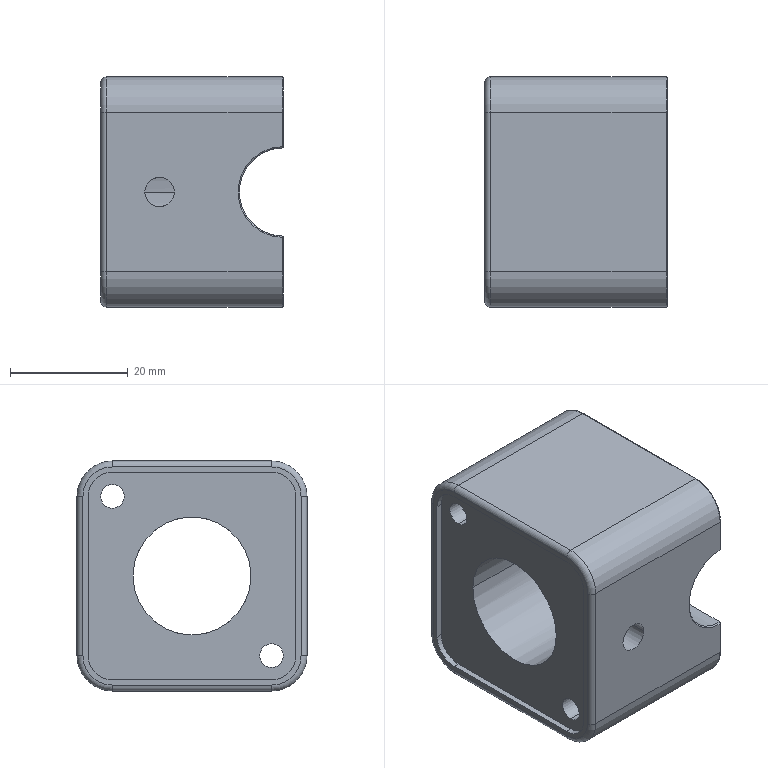NC program | NX | posted with a generic post | part box 31 x 39 x 39 mm
Whole program:
N10 G17 G21 G94 G90
(FACE_MILLING , TOOL : D50面刀)
N12 T01 M6
N14 G54
N16 G17 G0 G90 X-67.6 Y0. S3500 M3
N18 G43 Z13. H1
N20 Z3.
N22 G94 G1 Z0. F480.
N24 X-42.6
N26 X42.6 F800.
N28 X67.6
N30 Z3.
N32 G0 Z13.
N34 M5
(ADAPTIVE_MILLING , TOOL : D12C)
N36 T02 M6
N38 G54
N40 G17 G0 G90 X-31.788 Y-0.055 S6500 M3
N42 G43 Z10.1 H2
N44 Z-29.
N46 G94 G1 Z-32. F1200.
N48 X-30.034 Y-0.606 F2000.
N50 G3 X-28.621 Y-0.055 R1.22
N52 X-27.902 Y2.503 R6.631
N54 X-27.53 Y11.115 R77.337
N56 G2 X-27.476 Y19.739 R652.011
N58 X-24.339 Y24.645 R7.121
N60 X-18.3 Y26.893 R14.361
N62 X-9.325 Y27.446 R63.764
N64 G1 X-8.2 Y27.458
N66 X-7.075 Y27.467
N68 X-5.45 Y27.474
N70 X-3.45 Y27.48
N72 X-0.325 Y27.483
N74 X5.925 Y27.484
N76 X19.175 Y27.482
N78 X19.3 Y27.481
N80 X19.425 Y27.477
N82 X19.55 Y27.471
N84 X19.675 Y27.46
N86 G2 X24.607 Y24.368 R7.095
N88 X26.884 Y18.34 R14.24
N90 X27.443 Y9.741 R59.794
N92 G1 X27.454 Y8.866
N94 X27.465 Y7.741
N96 X27.473 Y6.491
N98 X27.48 Y4.741
N100 X27.485 Y2.491
N102 X27.488 Y-1.384
N104 X27.489 Y-11.509
N106 Y-19.259
N108 X27.485 Y-19.383
N110 X27.479 Y-19.508
N112 X27.47 Y-19.633
N114 G2 X24.401 Y-24.579 R7.07
N116 X18.256 Y-26.89 R14.307
N118 X9.906 Y-27.432 R59.459
N120 G1 X8.906 Y-27.445
N122 X7.781 Y-27.456
N124 X6.406 Y-27.465
N126 X4.656 Y-27.472
N128 X2.156 Y-27.477
N130 X-1.719 Y-27.48
N132 X-12.969 Y-27.481
N134 X-19.219 Y-27.482
N136 X-19.344 Y-27.48
N138 X-19.469 Y-27.474
N140 X-19.593 Y-27.466
N142 G2 X-24.482 Y-24.531 R6.979
N144 X-26.869 Y-18.418 R13.923
N146 X-27.442 Y-9.57 R60.624
N148 X-27.394 Y-2.323 R91.496
N150 G3 X-26.539 Y13.769 R130.767
N152 G2 X-26.388 Y17.386 R22.547
N154 X-21.818 Y23.656 R9.393
N156 X-14.847 Y25.904 R18.303
N158 X-4.743 Y26.438 R83.08
N160 G1 X-3.618 Y26.448
N162 X-2.118 Y26.457
N164 X-0.243 Y26.464
N166 X2.257 Y26.469
N168 X6.257 Y26.472
N170 X15.882
N172 G2 X23.312 Y22.305 R9.011
N174 X25.832 Y15.306 R16.91
N176 X26.435 Y5.208 R73.872
N178 G1 X26.448 Y3.958
N180 X26.457 Y2.708
N182 X26.465 Y1.083
N184 X26.471 Y-1.042
N186 X26.476 Y-4.042
N188 X26.478 Y-9.667
N190 G2 X26.439 Y-16.666 R198.924
N192 X22.175 Y-23.4 R9.126
N194 X15.149 Y-25.851 R17.286
N196 X5.048 Y-26.428 R76.941
N198 G1 X3.923 Y-26.439
N200 X2.549 Y-26.449
N202 X0.924 Y-26.457
N204 X-1.201 Y-26.463
N206 X-4.326 Y-26.468
N208 X-10.201 Y-26.47
N210 G2 X-16.7 Y-26.429 R163.076
N212 X-23.422 Y-22.143 R9.144
N214 X-25.842 Y-15.237 R17.24
N216 X-26.04 Y0.726 R70.302
N218 G3 X-25.583 Y13.777 R171.534
N220 G2 X-24.847 Y17.688 R13.664
N222 X-22.73 Y21.317 R13.93
N224 X-19.5 Y24.002 R13.93
N226 X-15.546 Y25.421 R13.93
N228 G1 X-13.527 Y25.598
N230 X-13.472 Y25.6
N232 X13.472
N234 X13.527 Y25.598
N236 G2 X17.585 Y24.885 R14.157
N238 X21.317 Y22.73 R13.76
N240 X24.002 Y19.5 R13.93
N242 X25.421 Y15.546 R13.93
N244 G1 X25.598 Y13.527
N246 X25.6 Y13.472
N248 Y-13.472
N250 X25.598 Y-13.527
N252 G2 X24.885 Y-17.585 R14.157
N254 X22.73 Y-21.317 R13.76
N256 X19.5 Y-24.002 R13.93
N258 X15.546 Y-25.421 R13.93
N260 G1 X13.527 Y-25.598
N262 X13.472 Y-25.6
N264 X-13.472
N266 X-13.527 Y-25.598
N268 G2 X-17.585 Y-24.885 R14.157
N270 X-21.317 Y-22.73 R13.76
N272 X-24.002 Y-19.5 R13.93
N274 X-25.421 Y-15.546 R13.93
N276 G1 X-25.598 Y-13.527
N278 X-25.6 Y-13.472
N280 Y13.472
N282 X-25.598 Y13.527
N284 X-25.5 Y14.648
N286 G3 X-26.643 Y15.964 R1.217
N288 G1 X-28.366 Y16.056
N290 Z-29.
N292 G0 Z10.1
(HOLE_MILLING , TOOL : D12C)
N294 X0. Y0.
N296 Z10.
N298 Z0.5
N300 G3 X1.9 Y1.9 R1.9 F300.
N302 X0. Y3.8 R1.9
N304 X0. Y3.8 Z-0.5 I0. J-3.8 F500.
N306 X0. Y3.8 Z-1.5 I0. J-3.8
N308 X0. Y3.8 Z-2.5 I0. J-3.8
N310 X0. Y3.8 Z-3.5 I0. J-3.8
N312 X0. Y3.8 Z-4.5 I0. J-3.8
N314 X0. Y3.8 Z-5.5 I0. J-3.8
N316 X0. Y3.8 Z-6.5 I0. J-3.8
N318 X0. Y3.8 Z-7.5 I0. J-3.8
N320 X0. Y3.8 Z-8.5 I0. J-3.8
N322 X0. Y3.8 Z-9.5 I0. J-3.8
N324 X0. Y3.8 Z-10.5 I0. J-3.8
N326 X0. Y3.8 Z-11.5 I0. J-3.8
N328 X0. Y3.8 Z-12.5 I0. J-3.8
N330 X0. Y3.8 Z-13.5 I0. J-3.8
N332 X0. Y3.8 Z-14.5 I0. J-3.8
N334 X0. Y3.8 Z-15.5 I0. J-3.8
N336 X0. Y3.8 Z-16.5 I0. J-3.8
N338 X0. Y3.8 Z-17.5 I0. J-3.8
N340 X0. Y3.8 Z-18.5 I0. J-3.8
N342 X0. Y3.8 Z-19.5 I0. J-3.8
N344 X0. Y3.8 Z-20.5 I0. J-3.8
N346 X0. Y3.8 Z-21.5 I0. J-3.8
N348 X0. Y3.8 Z-22.5 I0. J-3.8
N350 X0. Y3.8 Z-23.5 I0. J-3.8
N352 X0. Y3.8 Z-24.5 I0. J-3.8
N354 X0. Y3.8 Z-25.5 I0. J-3.8
N356 X0. Y3.8 Z-26.5 I0. J-3.8
N358 X0. Y3.8 Z-27.5 I0. J-3.8
N360 X0. Y3.8 Z-28.5 I0. J-3.8
N362 X0. Y3.8 Z-29.5 I0. J-3.8
N364 X0. Y3.8 Z-30.5 I0. J-3.8
N366 X0. Y3.8 Z-31.5 I0. J-3.8
N368 X-3.8 Y0. R3.8
N370 X0. Y3.8 R-3.8
N372 X-1.9 Y1.9 R1.9
N374 X0. Y0. R1.9
N376 G0 Z10.
(PLANAR_PROFILE , TOOL : D12C)
N378 X-28.5 Y-16.5 S3500
N380 Z-29.
N382 G1 Z-32. F800.
N384 G3 X-25.5 Y-13.5 R3.
N386 G1 Y13.5
N388 G2 X-13.5 Y25.5 R12.
N390 G1 X13.5
N392 G2 X25.5 Y13.5 R12.
N394 G1 Y-13.5
N396 G2 X13.5 Y-25.5 R12.
N398 G1 X-13.5
N400 G2 X-25.5 Y-13.5 R12.
N402 G3 X-28.5 Y-10.5 R3.
N404 G1 Z-29.
N406 G0 Z10.
(PLANAR_PROFILE_COPY , TOOL : D12C)
N408 X-1. Y-2.828 S4500
N410 Z-30.
N412 G1 Z-32. F300.
N414 Y-3.
N416 G3 X0. Y-4. R1.
N418 X4. Y0. R4.
N420 X0. Y-4. R-4.
N422 X1. Y-3. R1.
N424 G1 Y-2.828
N426 Z-30.
N428 G0 Z10.
N430 M5
(PLANAR_PROFILE_COPY_COPY , TOOL : D10点钻)
N432 T03 M6
N434 G54
N436 G17 G0 G90 X-1. Y-7.433 S3500 M3
N438 G43 Z10. H3
N440 Z0.5
N442 G94 G1 Z-1.5 F800.
N444 Y-7.5
N446 G3 X0. Y-8.5 R1.
N448 X8.5 Y0. R8.5
N450 X0. Y-8.5 R-8.5
N452 X1. Y-7.433 R1.002
N454 G1 Z0.5
N456 G0 Z10.
(DRILLING , TOOL : D10点钻)
N458 S1200
N460 X-13.5 Y13.5
N462 G43 Z3. H3
N464 G81 G99 Z-3.6 F250. R3.
N466 X13.5 Y-13.5
N468 G80
(DRILLING_COPY , TOOL : D10点钻)
N470 G81 X-13.5 Y-13.5 Z-2. F250. R3.
N472 X13.5 Y13.5
N474 G80
N476 M5
(DRILLING_COPY_1 , TOOL : D4.2钻头)
N478 T04 M6
N480 G54
N482 G17 G43 G0 G90 X-13.5 Y13.5 S2000 H4 M3
N484 Z3.
N486 G94 G83 G99 Z-33. F250. Q3. R3.
N488 X13.5 Y-13.5
N490 G80
N492 M5
(DRILLING_COPY_COPY , TOOL : D3.3钻头)
N494 T05 M6
N496 G54
N498 G17 G0 G90 X-13.5 Y-13.5 S1200 M3
N500 G43 Z3. H5
N502 G94 G81 G99 Z-11.5 F250. R3.
N504 X13.5 Y13.5
N506 G80
N508 M5
(HOLE_MILLING_1 , TOOL : D5精刀)
N510 T07 M6
N512 G54
N514 G17 G0 G90 X-13.5 Y13.5 S4500 M3
N516 G43 Z10. H7
N518 Z0.3
N520 G94 G3 X-12.95 Y14.05 R0.55 F800.
N522 X-13.5 Y14.6 R0.55
N524 X-13.5 Y14.6 Z-0.2 I0. J-1.1
N526 X-13.5 Y14.6 Z-0.7 I0. J-1.1
N528 X-13.5 Y14.6 Z-1.2 I0. J-1.1
N530 X-13.5 Y14.6 Z-1.7 I0. J-1.1
N532 X-13.5 Y14.6 Z-2.2 I0. J-1.1
N534 X-13.5 Y14.6 Z-2.7 I0. J-1.1
N536 X-13.5 Y14.6 Z-3.2 I0. J-1.1
N538 X-13.5 Y14.6 Z-3.7 I0. J-1.1
N540 X-13.5 Y14.6 Z-4.2 I0. J-1.1
N542 X-13.5 Y14.6 Z-4.7 I0. J-1.1
N544 X-13.5 Y14.6 Z-5.2 I0. J-1.1
N546 X-13.5 Y14.6 Z-5.7 I0. J-1.1
N548 X-13.5 Y14.6 Z-6.2 I0. J-1.1
N550 X-13.5 Y14.6 Z-6.7 I0. J-1.1
N552 X-13.5 Y14.6 Z-7.2 I0. J-1.1
N554 X-13.5 Y14.6 Z-7.7 I0. J-1.1
N556 X-13.5 Y14.6 Z-8.2 I0. J-1.1
N558 X-13.5 Y14.6 Z-8.7 I0. J-1.1
N560 X-13.5 Y14.6 Z-9.2 I0. J-1.1
N562 X-13.5 Y14.6 Z-9.7 I0. J-1.1
N564 X-12.853 Y12.61 Z-10. R-1.1
N566 X-12.61 Y14.147 R1.1
N568 X-12.853 Y12.61 R-1.1
N570 X-12.732 Y13.378 R0.55
N572 X-13.5 Y13.5 R0.55
N574 G0 Z10.
N576 X13.5 Y-13.5
N578 Z0.3
N580 G3 X14.05 Y-12.95 R0.55
N582 X13.5 Y-12.4 R0.55
N584 X13.5 Y-12.4 Z-0.2 I0. J-1.1
N586 X13.5 Y-12.4 Z-0.7 I0. J-1.1
N588 X13.5 Y-12.4 Z-1.2 I0. J-1.1
N590 X13.5 Y-12.4 Z-1.7 I0. J-1.1
N592 X13.5 Y-12.4 Z-2.2 I0. J-1.1
N594 X13.5 Y-12.4 Z-2.7 I0. J-1.1
N596 X13.5 Y-12.4 Z-3.2 I0. J-1.1
N598 X13.5 Y-12.4 Z-3.7 I0. J-1.1
N600 X13.5 Y-12.4 Z-4.2 I0. J-1.1
N602 X13.5 Y-12.4 Z-4.7 I0. J-1.1
N604 X13.5 Y-12.4 Z-5.2 I0. J-1.1
N606 X13.5 Y-12.4 Z-5.7 I0. J-1.1
N608 X13.5 Y-12.4 Z-6.2 I0. J-1.1
N610 X13.5 Y-12.4 Z-6.7 I0. J-1.1
N612 X13.5 Y-12.4 Z-7.2 I0. J-1.1
N614 X13.5 Y-12.4 Z-7.7 I0. J-1.1
N616 X13.5 Y-12.4 Z-8.2 I0. J-1.1
N618 X13.5 Y-12.4 Z-8.7 I0. J-1.1
N620 X13.5 Y-12.4 Z-9.2 I0. J-1.1
N622 X13.5 Y-12.4 Z-9.7 I0. J-1.1
N624 X14.147 Y-14.39 Z-10. R-1.1
N626 X14.39 Y-12.853 R1.1
N628 X14.147 Y-14.39 R-1.1
N630 X14.268 Y-13.622 R0.55
N632 X13.5 Y-13.5 R0.55
N634 G0 Z10.
N636 M5
(ZLEVEL_PROFILE , TOOL : R0.5)
N638 T08 M6
N640 G54
N642 G17 G0 G90 X-7.084 Y-19.774 S4500 M3
N644 G43 Z10. H8
N646 Z2.98
N648 G94 G1 Z-0.02 F1500.
N650 G3 X-7.546 Y-19.466 R0.5
N652 G1 X-13.5
N654 G2 X-19.466 Y-13.5 R5.966
N656 G1 Y13.5
N658 G2 X-13.5 Y19.466 R5.966
N660 G1 X-7.546
N662 X-7.555 Y19.502 Z-0.03
N664 X-7.564 Y19.533 Z-0.04
N666 X-13.5
N668 G3 X-19.533 Y13.5 R6.033
N670 G1 Y-13.5
N672 G3 X-13.5 Y-19.533 R6.033
N674 G1 X-7.564
N676 X-7.571 Y-19.56 Z-0.05
N678 X-7.578 Y-19.584 Z-0.06
N680 X-13.5
N682 G2 X-19.584 Y-13.5 R6.084
N684 G1 Y13.5
N686 G2 X-13.5 Y19.584 R6.084
N688 G1 X-7.578
N690 X-7.583 Y19.605 Z-0.07
N692 X-7.589 Y19.625 Z-0.08
N694 X-13.5
N696 G3 X-19.625 Y13.5 R6.125
N698 G1 Y-13.5
N700 G3 X-13.5 Y-19.625 R6.125
N702 G1 X-7.589
N704 X-7.598 Y-19.661 Z-0.1
N706 X-13.5
N708 G2 X-19.661 Y-13.5 R6.161
N710 G1 Y13.5
N712 G2 X-13.5 Y19.661 R6.161
N714 G1 X-7.598
N716 X-7.607 Y19.692 Z-0.12
N718 X-13.5
N720 G3 X-19.692 Y13.5 R6.192
N722 G1 Y-13.5
N724 G3 X-13.5 Y-19.692 R6.192
N726 G1 X-7.607
N728 X-7.615 Y-19.72 Z-0.14
N730 X-13.5
N732 G2 X-19.72 Y-13.5 R6.22
N734 G1 Y13.5
N736 G2 X-13.5 Y19.72 R6.22
N738 G1 X-7.615
N740 X-7.621 Y19.745 Z-0.16
N742 X-13.5
N744 G3 X-19.745 Y13.5 R6.245
N746 G1 Y-13.5
N748 G3 X-13.5 Y-19.745 R6.245
N750 G1 X-7.621
N752 X-7.628 Y-19.769 Z-0.18
N754 X-13.5
N756 G2 X-19.769 Y-13.5 R6.269
N758 G1 Y13.5
N760 G2 X-13.5 Y19.769 R6.269
N762 G1 X-7.628
N764 X-7.634 Y19.79 Z-0.2
N766 X-13.5
N768 G3 X-19.79 Y13.5 R6.29
N770 G1 Y-13.5
N772 G3 X-13.5 Y-19.79 R6.29
N774 G1 X-7.634
N776 G2 X-7.152 Y-20.157 R0.5
N778 G1 Z2.8
N780 G0 Z10.
N782 X7.084 Y19.774
N784 Z2.98
N786 G1 Z-0.02
N788 G3 X7.546 Y19.466 R0.5
N790 G1 X13.5
N792 G2 X19.466 Y13.5 R5.966
N794 G1 Y-13.5
N796 G2 X13.5 Y-19.466 R5.966
N798 G1 X7.546
N800 X7.555 Y-19.502 Z-0.03
N802 X7.564 Y-19.533 Z-0.04
N804 X13.5
N806 G3 X19.533 Y-13.5 R6.033
N808 G1 Y13.5
N810 G3 X13.5 Y19.533 R6.033
N812 G1 X7.564
N814 X7.571 Y19.56 Z-0.05
N816 X7.578 Y19.584 Z-0.06
N818 X13.5
N820 G2 X19.584 Y13.5 R6.084
N822 G1 Y-13.5
N824 G2 X13.5 Y-19.584 R6.084
N826 G1 X7.578
N828 X7.583 Y-19.605 Z-0.07
N830 X7.589 Y-19.625 Z-0.08
N832 X13.5
N834 G3 X19.625 Y-13.5 R6.125
N836 G1 Y13.5
N838 G3 X13.5 Y19.625 R6.125
N840 G1 X7.589
N842 X7.598 Y19.661 Z-0.1
N844 X13.5
N846 G2 X19.661 Y13.5 R6.161
N848 G1 Y-13.5
N850 G2 X13.5 Y-19.661 R6.161
N852 G1 X7.598
N854 X7.607 Y-19.692 Z-0.12
N856 X13.5
N858 G3 X19.692 Y-13.5 R6.192
N860 G1 Y13.5
N862 G3 X13.5 Y19.692 R6.192
N864 G1 X7.607
N866 X7.615 Y19.72 Z-0.14
N868 X13.5
N870 G2 X19.72 Y13.5 R6.22
N872 G1 Y-13.5
N874 G2 X13.5 Y-19.72 R6.22
N876 G1 X7.615
N878 X7.621 Y-19.745 Z-0.16
N880 X13.5
N882 G3 X19.745 Y-13.5 R6.245
N884 G1 Y13.5
N886 G3 X13.5 Y19.745 R6.245
N888 G1 X7.621
N890 X7.628 Y19.769 Z-0.18
N892 X13.5
N894 G2 X19.769 Y13.5 R6.269
N896 G1 Y-13.5
N898 G2 X13.5 Y-19.769 R6.269
N900 G1 X7.628
N902 X7.634 Y-19.79 Z-0.2
N904 X13.5
N906 G3 X19.79 Y-13.5 R6.29
N908 G1 Y13.5
N910 G3 X13.5 Y19.79 R6.29
N912 G1 X7.634
N914 G2 X7.152 Y20.157 R0.5
N916 G1 Z2.8
N918 G0 Z10.
N920 M5
(FACE_MILLING_COPY , TOOL : D50面刀)
N922 T01 M6
N924 G54
N926 G17 G0 G90 X-67.6 Y0. S3500 M3
N928 G43 Z11. H1
N930 Z3.05
N932 G94 G1 Z0.05 F480.
N934 X-42.6
N936 X42.6 F800.
N938 X67.6
N940 Z3.05
N942 G0 Z11.
(FACE_MILLING_COPY_COPY , TOOL : D50面刀)
N944 X-67.6
N946 Z3.
N948 G1 Z0. F480.
N950 X-42.6
N952 X42.6 F800.
N954 X67.6
N956 Z3.
N958 G0 Z11.
N960 M5
(PLANAR_MILL , TOOL : D5精刀)
N962 T07 M6
N964 G54
N966 G17 G0 G90 X0.059 Y0.081 S4500 M3
N968 G43 Z10.1 H7
N970 Z1.1
N972 G94 G1 Z-0.9 F600.
N974 X0. Y0.
N976 X2.5 F1000.
N978 Y2.5
N980 X-2.5
N982 Y-2.5
N984 X2.5
N986 Y0.
N988 X5.
N990 Y5.
N992 X-5.
N994 Y-5.
N996 X5.
N998 Y0.
N1000 X7.5
N1002 Y7.5
N1004 X-7.5
N1006 Y-7.5
N1008 X7.5
N1010 Y0.
N1012 X10.
N1014 Y10.
N1016 X-10.
N1018 Y-10.
N1020 X10.
N1022 Y0.
N1024 X12.5
N1026 Y12.5
N1028 X-12.5
N1030 Y-12.5
N1032 X12.5
N1034 Y0.
N1036 X15.
N1038 Y13.5
N1040 G3 X13.5 Y15. R1.5
N1042 G1 X-13.5
N1044 G3 X-15. Y13.5 R1.5
N1046 G1 Y-13.5
N1048 G3 X-13.5 Y-15. R1.5
N1050 G1 X13.5
N1052 G3 X15. Y-13.5 R1.5
N1054 G1 Y0.
N1056 X14.9
N1058 Z1.1
N1060 G0 Z10.1
(PLANAR_MILL_COPY , TOOL : D5精刀)
N1062 X-2. Y0.
N1064 Z10.
N1066 Z1.
N1068 G1 Z-1. F600.
N1070 X-2.1
N1072 Y-2.1
N1074 X2.1
N1076 Y2.1
N1078 X-2.1
N1080 Y0.
N1082 X-5.35
N1084 Y-5.35
N1086 X5.35
N1088 Y5.35
N1090 X-5.35
N1092 Y0.
N1094 X-8.6
N1096 Y-8.6
N1098 X8.6
N1100 Y8.6
N1102 X-8.6
N1104 Y0.
N1106 X-11.85
N1108 Y-11.85
N1110 X11.85
N1112 Y11.85
N1114 X-11.85
N1116 Y0.
N1118 X-15.1
N1120 Y-13.5
N1122 G3 X-13.5 Y-15.1 R1.6
N1124 G1 X13.5
N1126 G3 X15.1 Y-13.5 R1.6
N1128 G1 Y13.5
N1130 G3 X13.5 Y15.1 R1.6
N1132 G1 X-13.5
N1134 G3 X-15.1 Y13.5 R1.6
N1136 G1 Y0.
N1138 X-15.
N1140 Z1.
N1142 G0 Z10.
N1144 M5
(PLANAR_PROFILE_1 , TOOL : R0.5)
N1146 T08 M6
N1148 G54
N1150 G17 G0 G90 X-14.192 Y0.5 S4500 M3
N1152 G43 Z10. H8
N1154 Z2.7
N1156 G94 G1 Z-0.3 F800.
N1158 X-16.692
N1160 G3 X-17.192 Y0. R0.5
N1162 G1 Y-13.5
N1164 G3 X-13.5 Y-17.192 R3.692
N1166 G1 X13.5
N1168 G3 X17.192 Y-13.5 R3.692
N1170 G1 Y13.5
N1172 G3 X13.5 Y17.192 R3.692
N1174 G1 X-13.5
N1176 G3 X-17.192 Y13.5 R3.692
N1178 G1 Y0.
N1180 G3 X-16.692 Y-0.5 R0.5
N1182 G1 X-14.192
N1184 Z2.7
N1186 G0 Z10.
(ZLEVEL_PROFILE_COPY , TOOL : R0.5)
N1188 X-19.244
N1190 Z2.98
N1192 G1 Z-0.02 F1500.
N1194 G3 X-18.744 Y0. R0.5
N1196 G1 Y13.5
N1198 G2 X-13.5 Y18.744 R5.244
N1200 G1 X13.5
N1202 G2 X18.744 Y13.5 R5.244
N1204 G1 Y-13.5
N1206 G2 X13.5 Y-18.744 R5.244
N1208 G1 X-13.5
N1210 G2 X-18.744 Y-13.5 R5.244
N1212 G1 Y0.
N1214 X-18.798 Z-0.03
N1216 X-18.844 Z-0.04
N1218 Y-13.5
N1220 G3 X-13.5 Y-18.844 R5.344
N1222 G1 X13.5
N1224 G3 X18.844 Y-13.5 R5.344
N1226 G1 Y13.5
N1228 G3 X13.5 Y18.844 R5.344
N1230 G1 X-13.5
N1232 G3 X-18.844 Y13.5 R5.344
N1234 G1 Y0.
N1236 X-18.884 Z-0.05
N1238 X-18.92 Z-0.06
N1240 Y13.5
N1242 G2 X-13.5 Y18.92 R5.42
N1244 G1 X13.5
N1246 G2 X18.92 Y13.5 R5.42
N1248 G1 Y-13.5
N1250 G2 X13.5 Y-18.92 R5.42
N1252 G1 X-13.5
N1254 G2 X-18.92 Y-13.5 R5.42
N1256 G1 Y0.
N1258 X-18.953 Z-0.07
N1260 X-18.983 Z-0.08
N1262 Y-13.5
N1264 G3 X-13.5 Y-18.983 R5.483
N1266 G1 X13.5
N1268 G3 X18.983 Y-13.5 R5.483
N1270 G1 Y13.5
N1272 G3 X13.5 Y18.983 R5.483
N1274 G1 X-13.5
N1276 G3 X-18.983 Y13.5 R5.483
N1278 G1 Y0.
N1280 X-19.012 Z-0.09
N1282 X-19.039 Z-0.1
N1284 Y13.5
N1286 G2 X-13.5 Y19.039 R5.539
N1288 G1 X13.5
N1290 G2 X19.039 Y13.5 R5.539
N1292 G1 Y-13.5
N1294 G2 X13.5 Y-19.039 R5.539
N1296 G1 X-13.5
N1298 G2 X-19.039 Y-13.5 R5.539
N1300 G1 Y0.
N1302 X-19.064 Z-0.11
N1304 X-19.088 Z-0.12
N1306 Y-13.5
N1308 G3 X-13.5 Y-19.088 R5.588
N1310 G1 X13.5
N1312 G3 X19.088 Y-13.5 R5.588
N1314 G1 Y13.5
N1316 G3 X13.5 Y19.088 R5.588
N1318 G1 X-13.5
N1320 G3 X-19.088 Y13.5 R5.588
N1322 G1 Y0.
N1324 X-19.111 Z-0.13
N1326 X-19.133 Z-0.14
N1328 Y13.5
N1330 G2 X-13.5 Y19.133 R5.633
N1332 G1 X13.5
N1334 G2 X19.133 Y13.5 R5.633
N1336 G1 Y-13.5
N1338 G2 X13.5 Y-19.133 R5.633
N1340 G1 X-13.5
N1342 G2 X-19.133 Y-13.5 R5.633
N1344 G1 Y0.
N1346 X-19.154 Z-0.15
N1348 X-19.174 Z-0.16
N1350 Y-13.5
N1352 G3 X-13.5 Y-19.174 R5.674
N1354 G1 X13.5
N1356 G3 X19.174 Y-13.5 R5.674
N1358 G1 Y13.5
N1360 G3 X13.5 Y19.174 R5.674
N1362 G1 X-13.5
N1364 G3 X-19.174 Y13.5 R5.674
N1366 G1 Y0.
N1368 X-19.194 Z-0.17
N1370 X-19.212 Z-0.18
N1372 Y13.5
N1374 G2 X-13.5 Y19.212 R5.712
N1376 G1 X13.5
N1378 G2 X19.212 Y13.5 R5.712
N1380 G1 Y-13.5
N1382 G2 X13.5 Y-19.212 R5.712
N1384 G1 X-13.5
N1386 G2 X-19.212 Y-13.5 R5.712
N1388 G1 Y0.
N1390 X-19.231 Z-0.19
N1392 X-19.248 Z-0.2
N1394 Y-13.5
N1396 G3 X-13.5 Y-19.248 R5.748
N1398 G1 X13.5
N1400 G3 X19.248 Y-13.5 R5.748
N1402 G1 Y13.5
N1404 G3 X13.5 Y19.248 R5.748
N1406 G1 X-13.5
N1408 G3 X-19.248 Y13.5 R5.748
N1410 G1 Y0.
N1412 X-19.265 Z-0.21
N1414 X-19.282 Z-0.22
N1416 Y13.5
N1418 G2 X-13.5 Y19.282 R5.782
N1420 G1 X13.5
N1422 G2 X19.282 Y13.5 R5.782
N1424 G1 Y-13.5
N1426 G2 X13.5 Y-19.282 R5.782
N1428 G1 X-13.5
N1430 G2 X-19.282 Y-13.5 R5.782
N1432 G1 Y0.
N1434 X-19.298 Z-0.23
N1436 X-19.314 Z-0.24
N1438 Y-13.5
N1440 G3 X-13.5 Y-19.314 R5.814
N1442 G1 X13.5
N1444 G3 X19.314 Y-13.5 R5.814
N1446 G1 Y13.5
N1448 G3 X13.5 Y19.314 R5.814
N1450 G1 X-13.5
N1452 G3 X-19.314 Y13.5 R5.814
N1454 G1 Y0.
N1456 X-19.329 Z-0.25
N1458 X-19.344 Z-0.26
N1460 Y13.5
N1462 G2 X-13.5 Y19.344 R5.844
N1464 G1 X13.5
N1466 G2 X19.344 Y13.5 R5.844
N1468 G1 Y-13.5
N1470 G2 X13.5 Y-19.344 R5.844
N1472 G1 X-13.5
N1474 G2 X-19.344 Y-13.5 R5.844
N1476 G1 Y0.
N1478 X-19.359 Z-0.27
N1480 X-19.373 Z-0.28
N1482 Y-13.5
N1484 G3 X-13.5 Y-19.373 R5.873
N1486 G1 X13.5
N1488 G3 X19.373 Y-13.5 R5.873
N1490 G1 Y13.5
N1492 G3 X13.5 Y19.373 R5.873
N1494 G1 X-13.5
N1496 G3 X-19.373 Y13.5 R5.873
N1498 G1 Y0.
N1500 X-19.387 Z-0.29
N1502 X-19.4 Z-0.3
N1504 Y13.5
N1506 G2 X-13.5 Y19.4 R5.9
N1508 G1 X13.5
N1510 G2 X19.4 Y13.5 R5.9
N1512 G1 Y-13.5
N1514 G2 X13.5 Y-19.4 R5.9
N1516 G1 X-13.5
N1518 G2 X-19.4 Y-13.5 R5.9
N1520 G1 Y0.
N1522 X-19.413 Z-0.31
N1524 X-19.426 Z-0.32
N1526 Y-13.5
N1528 G3 X-13.5 Y-19.426 R5.926
N1530 G1 X13.5
N1532 G3 X19.426 Y-13.5 R5.926
N1534 G1 Y13.5
N1536 G3 X13.5 Y19.426 R5.926
N1538 G1 X-13.5
N1540 G3 X-19.426 Y13.5 R5.926
N1542 G1 Y0.
N1544 X-19.439 Z-0.33
N1546 X-19.451 Z-0.34
N1548 Y13.5
N1550 G2 X-13.5 Y19.451 R5.951
N1552 G1 X13.5
N1554 G2 X19.451 Y13.5 R5.951
N1556 G1 Y-13.5
N1558 G2 X13.5 Y-19.451 R5.951
N1560 G1 X-13.5
N1562 G2 X-19.451 Y-13.5 R5.951
N1564 G1 Y0.
N1566 X-19.463 Z-0.35
N1568 X-19.475 Z-0.36
N1570 Y-13.5
N1572 G3 X-13.5 Y-19.475 R5.975
N1574 G1 X13.5
N1576 G3 X19.475 Y-13.5 R5.975
N1578 G1 Y13.5
N1580 G3 X13.5 Y19.475 R5.975
N1582 G1 X-13.5
N1584 G3 X-19.475 Y13.5 R5.975
N1586 G1 Y0.
N1588 X-19.486 Z-0.37
N1590 X-19.498 Z-0.38
N1592 Y13.5
N1594 G2 X-13.5 Y19.498 R5.998
N1596 G1 X13.5
N1598 G2 X19.498 Y13.5 R5.998
N1600 G1 Y-13.5
N1602 G2 X13.5 Y-19.498 R5.998
N1604 G1 X-13.5
N1606 G2 X-19.498 Y-13.5 R5.998
N1608 G1 Y0.
N1610 X-19.509 Z-0.39
N1612 X-19.52 Z-0.4
N1614 Y-13.5
N1616 G3 X-13.5 Y-19.52 R6.02
N1618 G1 X13.5
N1620 G3 X19.52 Y-13.5 R6.02
N1622 G1 Y13.5
N1624 G3 X13.5 Y19.52 R6.02
N1626 G1 X-13.5
N1628 G3 X-19.52 Y13.5 R6.02
N1630 G1 Y0.
N1632 X-19.53 Z-0.41
N1634 X-19.541 Z-0.42
N1636 Y13.5
N1638 G2 X-13.5 Y19.541 R6.041
N1640 G1 X13.5
N1642 G2 X19.541 Y13.5 R6.041
N1644 G1 Y-13.5
N1646 G2 X13.5 Y-19.541 R6.041
N1648 G1 X-13.5
N1650 G2 X-19.541 Y-13.5 R6.041
N1652 G1 Y0.
N1654 X-19.551 Z-0.43
N1656 X-19.561 Z-0.44
N1658 Y-13.5
N1660 G3 X-13.5 Y-19.561 R6.061
N1662 G1 X13.5
N1664 G3 X19.561 Y-13.5 R6.061
N1666 G1 Y13.5
N1668 G3 X13.5 Y19.561 R6.061
N1670 G1 X-13.5
N1672 G3 X-19.561 Y13.5 R6.061
N1674 G1 Y0.
N1676 X-19.571 Z-0.45
N1678 X-19.581 Z-0.46
N1680 Y13.5
N1682 G2 X-13.5 Y19.581 R6.081
N1684 G1 X13.5
N1686 G2 X19.581 Y13.5 R6.081
N1688 G1 Y-13.5
N1690 G2 X13.5 Y-19.581 R6.081
N1692 G1 X-13.5
N1694 G2 X-19.581 Y-13.5 R6.081
N1696 G1 Y0.
N1698 X-19.59 Z-0.47
N1700 X-19.6 Z-0.48
N1702 Y-13.5
N1704 G3 X-13.5 Y-19.6 R6.1
N1706 G1 X13.5
N1708 G3 X19.6 Y-13.5 R6.1
N1710 G1 Y13.5
N1712 G3 X13.5 Y19.6 R6.1
N1714 G1 X-13.5
N1716 G3 X-19.6 Y13.5 R6.1
N1718 G1 Y0.
N1720 X-19.609 Z-0.49
N1722 X-19.618 Z-0.5
N1724 Y13.5
N1726 G2 X-13.5 Y19.618 R6.118
N1728 G1 X13.5
N1730 G2 X19.618 Y13.5 R6.118
N1732 G1 Y-13.5
N1734 G2 X13.5 Y-19.618 R6.118
N1736 G1 X-13.5
N1738 G2 X-19.618 Y-13.5 R6.118
N1740 G1 Y0.
N1742 X-19.627 Z-0.51
N1744 X-19.636 Z-0.52
N1746 Y-13.5
N1748 G3 X-13.5 Y-19.636 R6.136
N1750 G1 X13.5
N1752 G3 X19.636 Y-13.5 R6.136
N1754 G1 Y13.5
N1756 G3 X13.5 Y19.636 R6.136
N1758 G1 X-13.5
N1760 G3 X-19.636 Y13.5 R6.136
N1762 G1 Y0.
N1764 X-19.644 Z-0.53
N1766 X-19.653 Z-0.54
N1768 Y13.5
N1770 G2 X-13.5 Y19.653 R6.153
N1772 G1 X13.5
N1774 G2 X19.653 Y13.5 R6.153
N1776 G1 Y-13.5
N1778 G2 X13.5 Y-19.653 R6.153
N1780 G1 X-13.5
N1782 G2 X-19.653 Y-13.5 R6.153
N1784 G1 Y0.
N1786 X-19.661 Z-0.55
N1788 X-19.669 Z-0.56
N1790 Y-13.5
N1792 G3 X-13.5 Y-19.669 R6.169
N1794 G1 X13.5
N1796 G3 X19.669 Y-13.5 R6.169
N1798 G1 Y13.5
N1800 G3 X13.5 Y19.669 R6.169
N1802 G1 X-13.5
N1804 G3 X-19.669 Y13.5 R6.169
N1806 G1 Y0.
N1808 X-19.677 Z-0.57
N1810 X-19.685 Z-0.58
N1812 Y13.5
N1814 G2 X-13.5 Y19.685 R6.185
N1816 G1 X13.5
N1818 G2 X19.685 Y13.5 R6.185
N1820 G1 Y-13.5
N1822 G2 X13.5 Y-19.685 R6.185
N1824 G1 X-13.5
N1826 G2 X-19.685 Y-13.5 R6.185
N1828 G1 Y0.
N1830 X-19.692 Z-0.59
N1832 X-19.7 Z-0.6
N1834 Y-13.5
N1836 G3 X-13.5 Y-19.7 R6.2
N1838 G1 X13.5
N1840 G3 X19.7 Y-13.5 R6.2
N1842 G1 Y13.5
N1844 G3 X13.5 Y19.7 R6.2
N1846 G1 X-13.5
N1848 G3 X-19.7 Y13.5 R6.2
N1850 G1 Y0.
N1852 X-19.707 Z-0.61
N1854 X-19.715 Z-0.62
N1856 Y13.5
N1858 G2 X-13.5 Y19.715 R6.215
N1860 G1 X13.5
N1862 G2 X19.715 Y13.5 R6.215
N1864 G1 Y-13.5
N1866 G2 X13.5 Y-19.715 R6.215
N1868 G1 X-13.5
N1870 G2 X-19.715 Y-13.5 R6.215
N1872 G1 Y0.
N1874 X-19.722 Z-0.63
N1876 X-19.729 Z-0.64
N1878 Y-13.5
N1880 G3 X-13.5 Y-19.729 R6.229
N1882 G1 X13.5
N1884 G3 X19.729 Y-13.5 R6.229
N1886 G1 Y13.5
N1888 G3 X13.5 Y19.729 R6.229
N1890 G1 X-13.5
N1892 G3 X-19.729 Y13.5 R6.229
N1894 G1 Y0.
N1896 X-19.736 Z-0.65
N1898 X-19.743 Z-0.66
N1900 Y13.5
N1902 G2 X-13.5 Y19.743 R6.243
N1904 G1 X13.5
N1906 G2 X19.743 Y13.5 R6.243
N1908 G1 Y-13.5
N1910 G2 X13.5 Y-19.743 R6.243
N1912 G1 X-13.5
N1914 G2 X-19.743 Y-13.5 R6.243
N1916 G1 Y0.
N1918 X-19.749 Z-0.67
N1920 X-19.756 Z-0.68
N1922 Y-13.5
N1924 G3 X-13.5 Y-19.756 R6.256
N1926 G1 X13.5
N1928 G3 X19.756 Y-13.5 R6.256
N1930 G1 Y13.5
N1932 G3 X13.5 Y19.756 R6.256
N1934 G1 X-13.5
N1936 G3 X-19.756 Y13.5 R6.256
N1938 G1 Y0.
N1940 X-19.762 Z-0.69
N1942 X-19.769 Z-0.7
N1944 Y13.5
N1946 G2 X-13.5 Y19.769 R6.269
N1948 G1 X13.5
N1950 G2 X19.769 Y13.5 R6.269
N1952 G1 Y-13.5
N1954 G2 X13.5 Y-19.769 R6.269
N1956 G1 X-13.5
N1958 G2 X-19.769 Y-13.5 R6.269
N1960 G1 Y0.
N1962 X-19.775 Z-0.71
N1964 X-19.781 Z-0.72
N1966 Y-13.5
N1968 G3 X-13.5 Y-19.781 R6.281
N1970 G1 X13.5
N1972 G3 X19.781 Y-13.5 R6.281
N1974 G1 Y13.5
N1976 G3 X13.5 Y19.781 R6.281
N1978 G1 X-13.5
N1980 G3 X-19.781 Y13.5 R6.281
N1982 G1 Y0.
N1984 X-19.787 Z-0.73
N1986 X-19.793 Z-0.74
N1988 Y13.5
N1990 G2 X-13.5 Y19.793 R6.293
N1992 G1 X13.5
N1994 G2 X19.793 Y13.5 R6.293
N1996 G1 Y-13.5
N1998 G2 X13.5 Y-19.793 R6.293
N2000 G1 X-13.5
N2002 G2 X-19.793 Y-13.5 R6.293
N2004 G1 Y0.
N2006 X-19.799 Z-0.75
N2008 X-19.805 Z-0.76
N2010 Y-13.5
N2012 G3 X-13.5 Y-19.805 R6.305
N2014 G1 X13.5
N2016 G3 X19.805 Y-13.5 R6.305
N2018 G1 Y13.5
N2020 G3 X13.5 Y19.805 R6.305
N2022 G1 X-13.5
N2024 G3 X-19.805 Y13.5 R6.305
N2026 G1 Y0.
N2028 X-19.81 Z-0.77
N2030 X-19.816 Z-0.78
N2032 Y13.5
N2034 G2 X-13.5 Y19.816 R6.316
N2036 G1 X13.5
N2038 G2 X19.816 Y13.5 R6.316
N2040 G1 Y-13.5
N2042 G2 X13.5 Y-19.816 R6.316
N2044 G1 X-13.5
N2046 G2 X-19.816 Y-13.5 R6.316
N2048 G1 Y0.
N2050 X-19.821 Z-0.79
N2052 X-19.827 Z-0.8
N2054 Y-13.5
N2056 G3 X-13.5 Y-19.827 R6.327
N2058 G1 X13.5
N2060 G3 X19.827 Y-13.5 R6.327
N2062 G1 Y13.5
N2064 G3 X13.5 Y19.827 R6.327
N2066 G1 X-13.5
N2068 G3 X-19.827 Y13.5 R6.327
N2070 G1 Y0.
N2072 X-19.832 Z-0.81
N2074 X-19.837 Z-0.82
N2076 Y13.5
N2078 G2 X-13.5 Y19.837 R6.337
N2080 G1 X13.5
N2082 G2 X19.837 Y13.5 R6.337
N2084 G1 Y-13.5
N2086 G2 X13.5 Y-19.837 R6.337
N2088 G1 X-13.5
N2090 G2 X-19.837 Y-13.5 R6.337
N2092 G1 Y0.
N2094 X-19.842 Z-0.83
N2096 X-19.847 Z-0.84
N2098 Y-13.5
N2100 G3 X-13.5 Y-19.847 R6.347
N2102 G1 X13.5
N2104 G3 X19.847 Y-13.5 R6.347
N2106 G1 Y13.5
N2108 G3 X13.5 Y19.847 R6.347
N2110 G1 X-13.5
N2112 G3 X-19.847 Y13.5 R6.347
N2114 G1 Y0.
N2116 X-19.852 Z-0.85
N2118 X-19.857 Z-0.86
N2120 Y13.5
N2122 G2 X-13.5 Y19.857 R6.357
N2124 G1 X13.5
N2126 G2 X19.857 Y13.5 R6.357
N2128 G1 Y-13.5
N2130 G2 X13.5 Y-19.857 R6.357
N2132 G1 X-13.5
N2134 G2 X-19.857 Y-13.5 R6.357
N2136 G1 Y0.
N2138 X-19.861 Z-0.87
N2140 X-19.866 Z-0.88
N2142 Y-13.5
N2144 G3 X-13.5 Y-19.866 R6.366
N2146 G1 X13.5
N2148 G3 X19.866 Y-13.5 R6.366
N2150 G1 Y13.5
N2152 G3 X13.5 Y19.866 R6.366
N2154 G1 X-13.5
N2156 G3 X-19.866 Y13.5 R6.366
N2158 G1 Y0.
N2160 X-19.87 Z-0.89
N2162 X-19.875 Z-0.9
N2164 Y13.5
N2166 G2 X-13.5 Y19.875 R6.375
N2168 G1 X13.5
N2170 G2 X19.875 Y13.5 R6.375
N2172 G1 Y-13.5
N2174 G2 X13.5 Y-19.875 R6.375
N2176 G1 X-13.5
N2178 G2 X-19.875 Y-13.5 R6.375
N2180 G1 Y0.
N2182 X-19.879 Z-0.91
N2184 X-19.883 Z-0.92
N2186 Y-13.5
N2188 G3 X-13.5 Y-19.883 R6.383
N2190 G1 X13.5
N2192 G3 X19.883 Y-13.5 R6.383
N2194 G1 Y13.5
N2196 G3 X13.5 Y19.883 R6.383
N2198 G1 X-13.5
N2200 G3 X-19.883 Y13.5 R6.383
N2202 G1 Y0.
N2204 X-19.887 Z-0.93
N2206 X-19.892 Z-0.94
N2208 Y13.5
N2210 G2 X-13.5 Y19.892 R6.392
N2212 G1 X13.5
N2214 G2 X19.892 Y13.5 R6.392
N2216 G1 Y-13.5
N2218 G2 X13.5 Y-19.892 R6.392
N2220 G1 X-13.5
N2222 G2 X-19.892 Y-13.5 R6.392
N2224 G1 Y0.
N2226 X-19.896 Z-0.95
N2228 X-19.899 Z-0.96
N2230 Y-13.5
N2232 G3 X-13.5 Y-19.899 R6.399
N2234 G1 X13.5
N2236 G3 X19.899 Y-13.5 R6.399
N2238 G1 Y13.5
N2240 G3 X13.5 Y19.899 R6.399
N2242 G1 X-13.5
N2244 G3 X-19.899 Y13.5 R6.399
N2246 G1 Y0.
N2248 X-19.903 Z-0.97
N2250 X-19.907 Z-0.98
N2252 Y13.5
N2254 G2 X-13.5 Y19.907 R6.407
N2256 G1 X13.5
N2258 G2 X19.907 Y13.5 R6.407
N2260 G1 Y-13.5
N2262 G2 X13.5 Y-19.907 R6.407
N2264 G1 X-13.5
N2266 G2 X-19.907 Y-13.5 R6.407
N2268 G1 Y0.
N2270 X-19.911 Z-0.99
N2272 X-19.914 Z-1.
N2274 Y-13.5
N2276 G3 X-13.5 Y-19.914 R6.414
N2278 G1 X13.5
N2280 G3 X19.914 Y-13.5 R6.414
N2282 G1 Y13.5
N2284 G3 X13.5 Y19.914 R6.414
N2286 G1 X-13.5
N2288 G3 X-19.914 Y13.5 R6.414
N2290 G1 Y0.
N2292 G2 X-20.414 Y-0.5 R0.5
N2294 G1 Z2.
N2296 G0 Z10.
N2298 M5
(DRILLING_1 , TOOL : D10点钻)
N2300 T03 M6
N2302 G54
N2304 G17 G0 G90 X10. Y0. S1200 M3
N2306 G43 Z3. H3
N2308 G94 G81 G99 Z-2.5 F250. R3.
N2310 G80
N2312 M5
(DRILLING_1_COPY , TOOL : D4.2钻头)
N2314 T04 M6
N2316 G54
N2318 G17 G0 G90 X10. Y0. S1200 M3
N2320 G43 Z3. H4
N2322 G94 G81 G99 Z-13. F250. R3.
N2324 G80
N2326 M5
(DRILLING_1_COPY_COPY , TOOL : D5精刀)
N2328 T07 M6
N2330 G54
N2332 G17 G0 G90 X10. Y0. S1600 M3
N2334 G43 Z3. H7
N2336 G94 G81 G99 Z-11. F200. R3.
N2338 G80
N2340 M5
(HOLE_MILLING_2 , TOOL : D12C)
N2342 T02 M6
N2344 G54
N2346 G17 G0 G90 X31. Y0. S4500 M3
N2348 G43 Z9.8 H2
N2350 Z0.
N2352 G94 G3 X30.275 Y0.725 R0.725 F400.
N2354 X29.55 Y0. R0.725
N2356 X29.55 Y0. Z-0.5 I1.45 J0.
N2358 X29.55 Y0. Z-1. I1.45 J0.
N2360 X29.55 Y0. Z-1.5 I1.45 J0.
N2362 X29.55 Y0. Z-2. I1.45 J0.
N2364 X29.55 Y0. Z-2.5 I1.45 J0.
N2366 X29.55 Y0. Z-3. I1.45 J0.
N2368 X29.55 Y0. Z-3.5 I1.45 J0.
N2370 X29.55 Y0. Z-4. I1.45 J0.
N2372 X29.55 Y0. Z-4.5 I1.45 J0.
N2374 X29.55 Y0. Z-5. I1.45 J0.
N2376 X29.55 Y0. Z-5.5 I1.45 J0.
N2378 X29.55 Y0. Z-6. I1.45 J0.
N2380 X29.55 Y0. Z-6.5 I1.45 J0.
N2382 X29.55 Y0. Z-7. I1.45 J0.
N2384 X29.55 Y0. Z-7.5 I1.45 J0.
N2386 X29.55 Y0. Z-8. I1.45 J0.
N2388 X29.55 Y0. Z-8.5 I1.45 J0.
N2390 X29.55 Y0. Z-9. I1.45 J0.
N2392 X29.55 Y0. Z-9.5 I1.45 J0.
N2394 X29.55 Y0. Z-10. I1.45 J0.
N2396 X29.55 Y0. Z-10.5 I1.45 J0.
N2398 X29.55 Y0. Z-11. I1.45 J0.
N2400 X29.55 Y0. Z-11.5 I1.45 J0.
N2402 X29.55 Y0. Z-12. I1.45 J0.
N2404 X29.55 Y0. Z-12.5 I1.45 J0.
N2406 X29.55 Y0. Z-13. I1.45 J0.
N2408 X29.55 Y0. Z-13.5 I1.45 J0.
N2410 X29.55 Y0. Z-14. I1.45 J0.
N2412 X29.55 Y0. Z-14.5 I1.45 J0.
N2414 X29.55 Y0. Z-15. I1.45 J0.
N2416 X29.55 Y0. Z-15.5 I1.45 J0.
N2418 X29.55 Y0. Z-16. I1.45 J0.
N2420 X29.55 Y0. Z-16.5 I1.45 J0.
N2422 X29.55 Y0. Z-17. I1.45 J0.
N2424 X29.55 Y0. Z-17.5 I1.45 J0.
N2426 X29.55 Y0. Z-18. I1.45 J0.
N2428 X29.55 Y0. Z-18.5 I1.45 J0.
N2430 X29.55 Y0. Z-19. I1.45 J0.
N2432 X29.55 Y0. Z-19.5 I1.45 J0.
N2434 X29.55 Y0. Z-20. I1.45 J0.
N2436 X29.55 Y0. Z-20.5 I1.45 J0.
N2438 X29.55 Y0. Z-21. I1.45 J0.
N2440 X29.55 Y0. Z-21.5 I1.45 J0.
N2442 X29.55 Y0. Z-22. I1.45 J0.
N2444 X29.55 Y0. Z-22.5 I1.45 J0.
N2446 X29.55 Y0. Z-23. I1.45 J0.
N2448 X29.55 Y0. Z-23.5 I1.45 J0.
N2450 X29.55 Y0. Z-24. I1.45 J0.
N2452 X29.55 Y0. Z-24.5 I1.45 J0.
N2454 X29.55 Y0. Z-25. I1.45 J0.
N2456 X29.55 Y0. Z-25.5 I1.45 J0.
N2458 X29.55 Y0. Z-26. I1.45 J0.
N2460 X29.55 Y0. Z-26.5 I1.45 J0.
N2462 X29.55 Y0. Z-27. I1.45 J0.
N2464 X29.55 Y0. Z-27.5 I1.45 J0.
N2466 X29.55 Y0. Z-28. I1.45 J0.
N2468 X29.55 Y0. Z-28.5 I1.45 J0.
N2470 X29.55 Y0. Z-29. I1.45 J0.
N2472 X29.55 Y0. Z-29.5 I1.45 J0.
N2474 X29.55 Y0. Z-30. I1.45 J0.
N2476 X29.55 Y0. Z-30.5 I1.45 J0.
N2478 X29.55 Y0. Z-31. I1.45 J0.
N2480 X29.55 Y0. Z-31.5 I1.45 J0.
N2482 X29.55 Y0. Z-32. I1.45 J0.
N2484 X29.55 Y0. Z-32.5 I1.45 J0.
N2486 X29.55 Y0. Z-33. I1.45 J0.
N2488 X29.55 Y0. Z-33.5 I1.45 J0.
N2490 X29.55 Y0. Z-34. I1.45 J0.
N2492 X29.55 Y0. Z-34.5 I1.45 J0.
N2494 X29.55 Y0. Z-35. I1.45 J0.
N2496 X29.55 Y0. Z-35.5 I1.45 J0.
N2498 X29.55 Y0. Z-36. I1.45 J0.
N2500 X29.55 Y0. Z-36.5 I1.45 J0.
N2502 X29.55 Y0. Z-37. I1.45 J0.
N2504 X29.55 Y0. Z-37.5 I1.45 J0.
N2506 X29.55 Y0. Z-38. I1.45 J0.
N2508 X29.55 Y0. Z-38.5 I1.45 J0.
N2510 X29.55 Y0. Z-39. I1.45 J0.
N2512 X30.552 Y1.379 Z-39.4 R-1.45
N2514 X29.621 Y-0.448 R1.45
N2516 X30.552 Y1.379 R-1.45
N2518 X30.086 Y0.465 R0.725
N2520 X31. Y0. R0.725
N2522 G0 Z9.8
(HOLE_MILLING_2_COPY , TOOL : D12C)
N2524 Z-39.4
N2526 G3 X30.25 Y0.75 R0.75 F200.
N2528 X29.5 Y0. R0.75
N2530 X31. Y-1.5 R1.5
N2532 X29.5 Y0. R-1.5
N2534 X30.25 Y-0.75 R0.75
N2536 X31. Y0. R0.75
N2538 G0 Z9.8
N2540 M5
N2542 M2